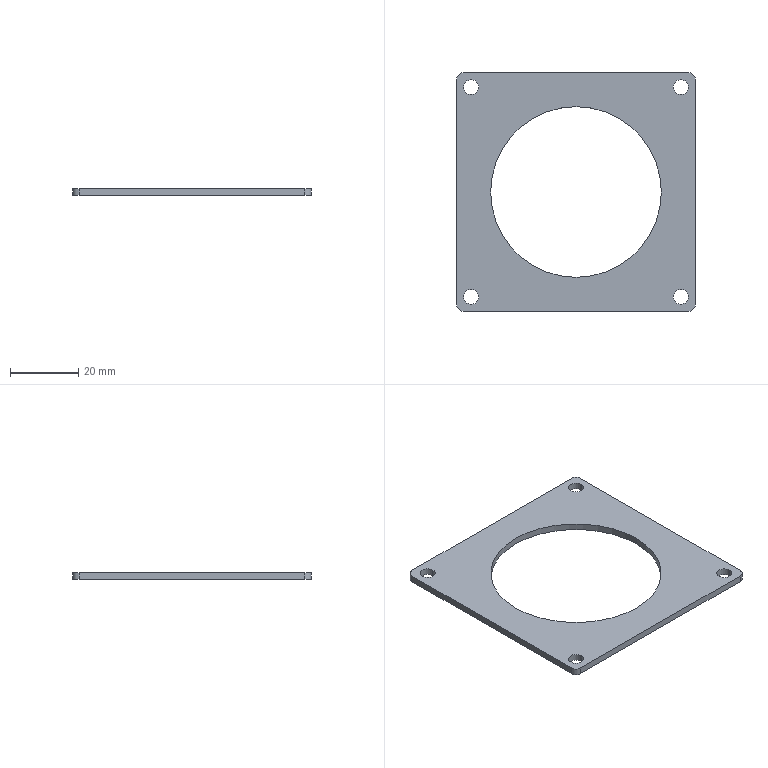Part | SolidWorks | features Cut 2, FlatPattern 1, SMBaseFlange 1, SheetMetal 1 | 1 solid | 20 faces | box 70 x 70 x 2 mm | volume 5744 mm3 | cylinder 14 | plane 6 | commonest cylinder face diameters 4.4 x8 4 x4 50 x2
STEP:
#1=CARTESIAN_POINT('',(-25.,0.,2.));
#2=VERTEX_POINT('',#1);
#3=CARTESIAN_POINT('',(25.,0.,2.));
#4=VERTEX_POINT('',#3);
#5=CARTESIAN_POINT('',(0.,0.,2.));
#6=DIRECTION('',(0.,0.,1.));
#7=DIRECTION('',(1.,0.,0.));
#8=AXIS2_PLACEMENT_3D('',#5,#6,#7);
#9=CIRCLE('',#8,25.);
#10=EDGE_CURVE('',#2,#4,#9,.T.);
#11=ORIENTED_EDGE('',*,*,#10,.T.);
#12=CARTESIAN_POINT('',(25.,0.,0.));
#13=VERTEX_POINT('',#12);
#14=CARTESIAN_POINT('',(25.,0.,10.));
#15=DIRECTION('',(0.,0.,-1.));
#16=VECTOR('',#15,1000.);
#17=LINE('',#14,#16);
#18=EDGE_CURVE('',#4,#13,#17,.T.);
#19=ORIENTED_EDGE('',*,*,#18,.T.);
#20=CARTESIAN_POINT('',(-25.,0.,0.));
#21=VERTEX_POINT('',#20);
#22=CARTESIAN_POINT('',(0.,0.,0.));
#23=DIRECTION('',(0.,0.,-1.));
#24=DIRECTION('',(-1.,0.,0.));
#25=AXIS2_PLACEMENT_3D('',#22,#23,#24);
#26=CIRCLE('',#25,25.);
#27=EDGE_CURVE('',#13,#21,#26,.T.);
#28=ORIENTED_EDGE('',*,*,#27,.T.);
#29=CARTESIAN_POINT('',(-25.,0.,10.));
#30=DIRECTION('',(0.,0.,-1.));
#31=VECTOR('',#30,1000.);
#32=LINE('',#29,#31);
#33=EDGE_CURVE('',#2,#21,#32,.T.);
#34=ORIENTED_EDGE('',*,*,#33,.F.);
#35=EDGE_LOOP('',(#11,#19,#28,#34));
#36=FACE_OUTER_BOUND('',#35,.T.);
#37=CARTESIAN_POINT('',(0.,0.,10.));
#38=DIRECTION('',(0.,0.,-1.));
#39=DIRECTION('',(-1.,0.,0.));
#40=AXIS2_PLACEMENT_3D('',#37,#38,#39);
#41=CYLINDRICAL_SURFACE('',#40,25.);
#42=ADVANCED_FACE('',(#36),#41,.F.);
#43=CARTESIAN_POINT('',(28.55,-30.75,2.));
#44=VERTEX_POINT('',#43);
#45=CARTESIAN_POINT('',(32.95,-30.75,2.));
#46=VERTEX_POINT('',#45);
#47=CARTESIAN_POINT('',(30.75,-30.75,2.));
#48=DIRECTION('',(0.,0.,1.));
#49=DIRECTION('',(1.,0.,0.));
#50=AXIS2_PLACEMENT_3D('',#47,#48,#49);
#51=CIRCLE('',#50,2.2);
#52=EDGE_CURVE('',#44,#46,#51,.T.);
#53=ORIENTED_EDGE('',*,*,#52,.T.);
#54=CARTESIAN_POINT('',(32.95,-30.75,0.));
#55=VERTEX_POINT('',#54);
#56=CARTESIAN_POINT('',(32.95,-30.75,10.));
#57=DIRECTION('',(0.,0.,-1.));
#58=VECTOR('',#57,1000.);
#59=LINE('',#56,#58);
#60=EDGE_CURVE('',#46,#55,#59,.T.);
#61=ORIENTED_EDGE('',*,*,#60,.T.);
#62=CARTESIAN_POINT('',(28.55,-30.75,0.));
#63=VERTEX_POINT('',#62);
#64=CARTESIAN_POINT('',(30.75,-30.75,0.));
#65=DIRECTION('',(0.,0.,-1.));
#66=DIRECTION('',(-1.,0.,0.));
#67=AXIS2_PLACEMENT_3D('',#64,#65,#66);
#68=CIRCLE('',#67,2.2);
#69=EDGE_CURVE('',#55,#63,#68,.T.);
#70=ORIENTED_EDGE('',*,*,#69,.T.);
#71=CARTESIAN_POINT('',(28.55,-30.75,10.));
#72=DIRECTION('',(0.,0.,-1.));
#73=VECTOR('',#72,1000.);
#74=LINE('',#71,#73);
#75=EDGE_CURVE('',#44,#63,#74,.T.);
#76=ORIENTED_EDGE('',*,*,#75,.F.);
#77=EDGE_LOOP('',(#53,#61,#70,#76));
#78=FACE_OUTER_BOUND('',#77,.T.);
#79=CARTESIAN_POINT('',(30.75,-30.75,10.));
#80=DIRECTION('',(0.,0.,-1.));
#81=DIRECTION('',(-1.,0.,0.));
#82=AXIS2_PLACEMENT_3D('',#79,#80,#81);
#83=CYLINDRICAL_SURFACE('',#82,2.2);
#84=ADVANCED_FACE('',(#78),#83,.F.);
#85=CARTESIAN_POINT('',(28.55,30.75,2.));
#86=VERTEX_POINT('',#85);
#87=CARTESIAN_POINT('',(32.95,30.75,2.));
#88=VERTEX_POINT('',#87);
#89=CARTESIAN_POINT('',(30.75,30.75,2.));
#90=DIRECTION('',(0.,0.,1.));
#91=DIRECTION('',(1.,0.,0.));
#92=AXIS2_PLACEMENT_3D('',#89,#90,#91);
#93=CIRCLE('',#92,2.2);
#94=EDGE_CURVE('',#86,#88,#93,.T.);
#95=ORIENTED_EDGE('',*,*,#94,.T.);
#96=CARTESIAN_POINT('',(32.95,30.75,0.));
#97=VERTEX_POINT('',#96);
#98=CARTESIAN_POINT('',(32.95,30.75,10.));
#99=DIRECTION('',(0.,0.,-1.));
#100=VECTOR('',#99,1000.);
#101=LINE('',#98,#100);
#102=EDGE_CURVE('',#88,#97,#101,.T.);
#103=ORIENTED_EDGE('',*,*,#102,.T.);
#104=CARTESIAN_POINT('',(28.55,30.75,0.));
#105=VERTEX_POINT('',#104);
#106=CARTESIAN_POINT('',(30.75,30.75,0.));
#107=DIRECTION('',(0.,0.,-1.));
#108=DIRECTION('',(-1.,0.,0.));
#109=AXIS2_PLACEMENT_3D('',#106,#107,#108);
#110=CIRCLE('',#109,2.2);
#111=EDGE_CURVE('',#97,#105,#110,.T.);
#112=ORIENTED_EDGE('',*,*,#111,.T.);
#113=CARTESIAN_POINT('',(28.55,30.75,10.));
#114=DIRECTION('',(0.,0.,-1.));
#115=VECTOR('',#114,1000.);
#116=LINE('',#113,#115);
#117=EDGE_CURVE('',#86,#105,#116,.T.);
#118=ORIENTED_EDGE('',*,*,#117,.F.);
#119=EDGE_LOOP('',(#95,#103,#112,#118));
#120=FACE_OUTER_BOUND('',#119,.T.);
#121=CARTESIAN_POINT('',(30.75,30.75,10.));
#122=DIRECTION('',(0.,0.,-1.));
#123=DIRECTION('',(-1.,0.,0.));
#124=AXIS2_PLACEMENT_3D('',#121,#122,#123);
#125=CYLINDRICAL_SURFACE('',#124,2.2);
#126=ADVANCED_FACE('',(#120),#125,.F.);
#127=CARTESIAN_POINT('',(-32.95,30.75,2.));
#128=VERTEX_POINT('',#127);
#129=CARTESIAN_POINT('',(-28.55,30.75,2.));
#130=VERTEX_POINT('',#129);
#131=CARTESIAN_POINT('',(-30.75,30.75,2.));
#132=DIRECTION('',(0.,0.,1.));
#133=DIRECTION('',(1.,0.,0.));
#134=AXIS2_PLACEMENT_3D('',#131,#132,#133);
#135=CIRCLE('',#134,2.2);
#136=EDGE_CURVE('',#128,#130,#135,.T.);
#137=ORIENTED_EDGE('',*,*,#136,.T.);
#138=CARTESIAN_POINT('',(-28.55,30.75,0.));
#139=VERTEX_POINT('',#138);
#140=CARTESIAN_POINT('',(-28.55,30.75,10.));
#141=DIRECTION('',(0.,0.,-1.));
#142=VECTOR('',#141,1000.);
#143=LINE('',#140,#142);
#144=EDGE_CURVE('',#130,#139,#143,.T.);
#145=ORIENTED_EDGE('',*,*,#144,.T.);
#146=CARTESIAN_POINT('',(-32.95,30.75,0.));
#147=VERTEX_POINT('',#146);
#148=CARTESIAN_POINT('',(-30.75,30.75,0.));
#149=DIRECTION('',(0.,0.,-1.));
#150=DIRECTION('',(-1.,0.,0.));
#151=AXIS2_PLACEMENT_3D('',#148,#149,#150);
#152=CIRCLE('',#151,2.2);
#153=EDGE_CURVE('',#139,#147,#152,.T.);
#154=ORIENTED_EDGE('',*,*,#153,.T.);
#155=CARTESIAN_POINT('',(-32.95,30.75,10.));
#156=DIRECTION('',(0.,0.,-1.));
#157=VECTOR('',#156,1000.);
#158=LINE('',#155,#157);
#159=EDGE_CURVE('',#128,#147,#158,.T.);
#160=ORIENTED_EDGE('',*,*,#159,.F.);
#161=EDGE_LOOP('',(#137,#145,#154,#160));
#162=FACE_OUTER_BOUND('',#161,.T.);
#163=CARTESIAN_POINT('',(-30.75,30.75,10.));
#164=DIRECTION('',(0.,0.,-1.));
#165=DIRECTION('',(-1.,0.,0.));
#166=AXIS2_PLACEMENT_3D('',#163,#164,#165);
#167=CYLINDRICAL_SURFACE('',#166,2.2);
#168=ADVANCED_FACE('',(#162),#167,.F.);
#169=CARTESIAN_POINT('',(-32.95,-30.75,2.));
#170=VERTEX_POINT('',#169);
#171=CARTESIAN_POINT('',(-28.55,-30.75,2.));
#172=VERTEX_POINT('',#171);
#173=CARTESIAN_POINT('',(-30.75,-30.75,2.));
#174=DIRECTION('',(0.,0.,1.));
#175=DIRECTION('',(1.,0.,0.));
#176=AXIS2_PLACEMENT_3D('',#173,#174,#175);
#177=CIRCLE('',#176,2.2);
#178=EDGE_CURVE('',#170,#172,#177,.T.);
#179=ORIENTED_EDGE('',*,*,#178,.T.);
#180=CARTESIAN_POINT('',(-28.55,-30.75,0.));
#181=VERTEX_POINT('',#180);
#182=CARTESIAN_POINT('',(-28.55,-30.75,10.));
#183=DIRECTION('',(0.,0.,-1.));
#184=VECTOR('',#183,1000.);
#185=LINE('',#182,#184);
#186=EDGE_CURVE('',#172,#181,#185,.T.);
#187=ORIENTED_EDGE('',*,*,#186,.T.);
#188=CARTESIAN_POINT('',(-32.95,-30.75,0.));
#189=VERTEX_POINT('',#188);
#190=CARTESIAN_POINT('',(-30.75,-30.75,0.));
#191=DIRECTION('',(0.,0.,-1.));
#192=DIRECTION('',(-1.,0.,0.));
#193=AXIS2_PLACEMENT_3D('',#190,#191,#192);
#194=CIRCLE('',#193,2.2);
#195=EDGE_CURVE('',#181,#189,#194,.T.);
#196=ORIENTED_EDGE('',*,*,#195,.T.);
#197=CARTESIAN_POINT('',(-32.95,-30.75,10.));
#198=DIRECTION('',(0.,0.,-1.));
#199=VECTOR('',#198,1000.);
#200=LINE('',#197,#199);
#201=EDGE_CURVE('',#170,#189,#200,.T.);
#202=ORIENTED_EDGE('',*,*,#201,.F.);
#203=EDGE_LOOP('',(#179,#187,#196,#202));
#204=FACE_OUTER_BOUND('',#203,.T.);
#205=CARTESIAN_POINT('',(-30.75,-30.75,10.));
#206=DIRECTION('',(0.,0.,-1.));
#207=DIRECTION('',(-1.,0.,0.));
#208=AXIS2_PLACEMENT_3D('',#205,#206,#207);
#209=CYLINDRICAL_SURFACE('',#208,2.2);
#210=ADVANCED_FACE('',(#204),#209,.F.);
#211=CARTESIAN_POINT('',(-35.,-33.,0.));
#212=VERTEX_POINT('',#211);
#213=CARTESIAN_POINT('',(-33.,-35.,0.));
#214=VERTEX_POINT('',#213);
#215=CARTESIAN_POINT('',(-33.,-33.,0.));
#216=DIRECTION('',(0.,0.,1.));
#217=DIRECTION('',(1.,0.,0.));
#218=AXIS2_PLACEMENT_3D('',#215,#216,#217);
#219=CIRCLE('',#218,2.);
#220=EDGE_CURVE('',#212,#214,#219,.T.);
#221=ORIENTED_EDGE('',*,*,#220,.T.);
#222=CARTESIAN_POINT('',(-33.,-35.,2.));
#223=VERTEX_POINT('',#222);
#224=CARTESIAN_POINT('',(-33.,-35.,2.));
#225=DIRECTION('',(0.,0.,-1.));
#226=VECTOR('',#225,1000.);
#227=LINE('',#224,#226);
#228=EDGE_CURVE('',#223,#214,#227,.T.);
#229=ORIENTED_EDGE('',*,*,#228,.F.);
#230=CARTESIAN_POINT('',(-35.,-33.,2.));
#231=VERTEX_POINT('',#230);
#232=CARTESIAN_POINT('',(-33.,-33.,2.));
#233=DIRECTION('',(0.,0.,1.));
#234=DIRECTION('',(1.,0.,0.));
#235=AXIS2_PLACEMENT_3D('',#232,#233,#234);
#236=CIRCLE('',#235,2.);
#237=EDGE_CURVE('',#231,#223,#236,.T.);
#238=ORIENTED_EDGE('',*,*,#237,.F.);
#239=CARTESIAN_POINT('',(-35.,-33.,2.));
#240=DIRECTION('',(0.,0.,-1.));
#241=VECTOR('',#240,1000.);
#242=LINE('',#239,#241);
#243=EDGE_CURVE('',#231,#212,#242,.T.);
#244=ORIENTED_EDGE('',*,*,#243,.T.);
#245=EDGE_LOOP('',(#221,#229,#238,#244));
#246=FACE_OUTER_BOUND('',#245,.T.);
#247=CARTESIAN_POINT('',(-33.,-33.,2.));
#248=DIRECTION('',(0.,0.,-1.));
#249=DIRECTION('',(-1.,0.,0.));
#250=AXIS2_PLACEMENT_3D('',#247,#248,#249);
#251=CYLINDRICAL_SURFACE('',#250,2.);
#252=ADVANCED_FACE('',(#246),#251,.T.);
#253=CARTESIAN_POINT('',(33.,-35.,0.));
#254=VERTEX_POINT('',#253);
#255=CARTESIAN_POINT('',(33.,-35.,0.));
#256=DIRECTION('',(1.,0.,0.));
#257=VECTOR('',#256,1000.);
#258=LINE('',#255,#257);
#259=EDGE_CURVE('',#214,#254,#258,.T.);
#260=ORIENTED_EDGE('',*,*,#259,.T.);
#261=CARTESIAN_POINT('',(33.,-35.,2.));
#262=VERTEX_POINT('',#261);
#263=CARTESIAN_POINT('',(33.,-35.,2.));
#264=DIRECTION('',(0.,0.,-1.));
#265=VECTOR('',#264,1000.);
#266=LINE('',#263,#265);
#267=EDGE_CURVE('',#262,#254,#266,.T.);
#268=ORIENTED_EDGE('',*,*,#267,.F.);
#269=CARTESIAN_POINT('',(33.,-35.,2.));
#270=DIRECTION('',(1.,0.,0.));
#271=VECTOR('',#270,1000.);
#272=LINE('',#269,#271);
#273=EDGE_CURVE('',#223,#262,#272,.T.);
#274=ORIENTED_EDGE('',*,*,#273,.F.);
#275=ORIENTED_EDGE('',*,*,#228,.T.);
#276=EDGE_LOOP('',(#260,#268,#274,#275));
#277=FACE_OUTER_BOUND('',#276,.T.);
#278=CARTESIAN_POINT('',(33.,-35.,2.));
#279=DIRECTION('',(0.,1.,0.));
#280=DIRECTION('',(0.,0.,1.));
#281=AXIS2_PLACEMENT_3D('',#278,#279,#280);
#282=PLANE('',#281);
#283=ADVANCED_FACE('',(#277),#282,.F.);
#284=CARTESIAN_POINT('',(35.,-33.,0.));
#285=VERTEX_POINT('',#284);
#286=CARTESIAN_POINT('',(33.,-33.,0.));
#287=DIRECTION('',(0.,0.,1.));
#288=DIRECTION('',(1.,0.,0.));
#289=AXIS2_PLACEMENT_3D('',#286,#287,#288);
#290=CIRCLE('',#289,2.);
#291=EDGE_CURVE('',#254,#285,#290,.T.);
#292=ORIENTED_EDGE('',*,*,#291,.T.);
#293=CARTESIAN_POINT('',(35.,-33.,2.));
#294=VERTEX_POINT('',#293);
#295=CARTESIAN_POINT('',(35.,-33.,2.));
#296=DIRECTION('',(0.,0.,-1.));
#297=VECTOR('',#296,1000.);
#298=LINE('',#295,#297);
#299=EDGE_CURVE('',#294,#285,#298,.T.);
#300=ORIENTED_EDGE('',*,*,#299,.F.);
#301=CARTESIAN_POINT('',(33.,-33.,2.));
#302=DIRECTION('',(0.,0.,1.));
#303=DIRECTION('',(1.,0.,0.));
#304=AXIS2_PLACEMENT_3D('',#301,#302,#303);
#305=CIRCLE('',#304,2.);
#306=EDGE_CURVE('',#262,#294,#305,.T.);
#307=ORIENTED_EDGE('',*,*,#306,.F.);
#308=ORIENTED_EDGE('',*,*,#267,.T.);
#309=EDGE_LOOP('',(#292,#300,#307,#308));
#310=FACE_OUTER_BOUND('',#309,.T.);
#311=CARTESIAN_POINT('',(33.,-33.,2.));
#312=DIRECTION('',(0.,0.,-1.));
#313=DIRECTION('',(-1.,0.,0.));
#314=AXIS2_PLACEMENT_3D('',#311,#312,#313);
#315=CYLINDRICAL_SURFACE('',#314,2.);
#316=ADVANCED_FACE('',(#310),#315,.T.);
#317=CARTESIAN_POINT('',(35.,33.,0.));
#318=VERTEX_POINT('',#317);
#319=CARTESIAN_POINT('',(35.,33.,0.));
#320=DIRECTION('',(0.,1.,0.));
#321=VECTOR('',#320,1000.);
#322=LINE('',#319,#321);
#323=EDGE_CURVE('',#285,#318,#322,.T.);
#324=ORIENTED_EDGE('',*,*,#323,.T.);
#325=CARTESIAN_POINT('',(35.,33.,2.));
#326=VERTEX_POINT('',#325);
#327=CARTESIAN_POINT('',(35.,33.,2.));
#328=DIRECTION('',(0.,0.,-1.));
#329=VECTOR('',#328,1000.);
#330=LINE('',#327,#329);
#331=EDGE_CURVE('',#326,#318,#330,.T.);
#332=ORIENTED_EDGE('',*,*,#331,.F.);
#333=CARTESIAN_POINT('',(35.,33.,2.));
#334=DIRECTION('',(0.,1.,0.));
#335=VECTOR('',#334,1000.);
#336=LINE('',#333,#335);
#337=EDGE_CURVE('',#294,#326,#336,.T.);
#338=ORIENTED_EDGE('',*,*,#337,.F.);
#339=ORIENTED_EDGE('',*,*,#299,.T.);
#340=EDGE_LOOP('',(#324,#332,#338,#339));
#341=FACE_OUTER_BOUND('',#340,.T.);
#342=CARTESIAN_POINT('',(35.,33.,2.));
#343=DIRECTION('',(-1.,0.,0.));
#344=DIRECTION('',(0.,0.,1.));
#345=AXIS2_PLACEMENT_3D('',#342,#343,#344);
#346=PLANE('',#345);
#347=ADVANCED_FACE('',(#341),#346,.F.);
#348=CARTESIAN_POINT('',(33.,35.,0.));
#349=VERTEX_POINT('',#348);
#350=CARTESIAN_POINT('',(33.,33.,0.));
#351=DIRECTION('',(0.,0.,1.));
#352=DIRECTION('',(1.,0.,0.));
#353=AXIS2_PLACEMENT_3D('',#350,#351,#352);
#354=CIRCLE('',#353,2.);
#355=EDGE_CURVE('',#318,#349,#354,.T.);
#356=ORIENTED_EDGE('',*,*,#355,.T.);
#357=CARTESIAN_POINT('',(33.,35.,2.));
#358=VERTEX_POINT('',#357);
#359=CARTESIAN_POINT('',(33.,35.,2.));
#360=DIRECTION('',(0.,0.,-1.));
#361=VECTOR('',#360,1000.);
#362=LINE('',#359,#361);
#363=EDGE_CURVE('',#358,#349,#362,.T.);
#364=ORIENTED_EDGE('',*,*,#363,.F.);
#365=CARTESIAN_POINT('',(33.,33.,2.));
#366=DIRECTION('',(0.,0.,1.));
#367=DIRECTION('',(1.,0.,0.));
#368=AXIS2_PLACEMENT_3D('',#365,#366,#367);
#369=CIRCLE('',#368,2.);
#370=EDGE_CURVE('',#326,#358,#369,.T.);
#371=ORIENTED_EDGE('',*,*,#370,.F.);
#372=ORIENTED_EDGE('',*,*,#331,.T.);
#373=EDGE_LOOP('',(#356,#364,#371,#372));
#374=FACE_OUTER_BOUND('',#373,.T.);
#375=CARTESIAN_POINT('',(33.,33.,2.));
#376=DIRECTION('',(0.,0.,-1.));
#377=DIRECTION('',(-1.,0.,0.));
#378=AXIS2_PLACEMENT_3D('',#375,#376,#377);
#379=CYLINDRICAL_SURFACE('',#378,2.);
#380=ADVANCED_FACE('',(#374),#379,.T.);
#381=CARTESIAN_POINT('',(-33.,35.,0.));
#382=VERTEX_POINT('',#381);
#383=CARTESIAN_POINT('',(-33.,35.,0.));
#384=DIRECTION('',(-1.,0.,0.));
#385=VECTOR('',#384,1000.);
#386=LINE('',#383,#385);
#387=EDGE_CURVE('',#349,#382,#386,.T.);
#388=ORIENTED_EDGE('',*,*,#387,.T.);
#389=CARTESIAN_POINT('',(-33.,35.,2.));
#390=VERTEX_POINT('',#389);
#391=CARTESIAN_POINT('',(-33.,35.,2.));
#392=DIRECTION('',(0.,0.,-1.));
#393=VECTOR('',#392,1000.);
#394=LINE('',#391,#393);
#395=EDGE_CURVE('',#390,#382,#394,.T.);
#396=ORIENTED_EDGE('',*,*,#395,.F.);
#397=CARTESIAN_POINT('',(-33.,35.,2.));
#398=DIRECTION('',(-1.,0.,0.));
#399=VECTOR('',#398,1000.);
#400=LINE('',#397,#399);
#401=EDGE_CURVE('',#358,#390,#400,.T.);
#402=ORIENTED_EDGE('',*,*,#401,.F.);
#403=ORIENTED_EDGE('',*,*,#363,.T.);
#404=EDGE_LOOP('',(#388,#396,#402,#403));
#405=FACE_OUTER_BOUND('',#404,.T.);
#406=CARTESIAN_POINT('',(-33.,35.,2.));
#407=DIRECTION('',(0.,-1.,0.));
#408=DIRECTION('',(0.,0.,-1.));
#409=AXIS2_PLACEMENT_3D('',#406,#407,#408);
#410=PLANE('',#409);
#411=ADVANCED_FACE('',(#405),#410,.F.);
#412=CARTESIAN_POINT('',(-35.,33.,0.));
#413=VERTEX_POINT('',#412);
#414=CARTESIAN_POINT('',(-33.,33.,0.));
#415=DIRECTION('',(0.,0.,1.));
#416=DIRECTION('',(1.,0.,0.));
#417=AXIS2_PLACEMENT_3D('',#414,#415,#416);
#418=CIRCLE('',#417,2.);
#419=EDGE_CURVE('',#382,#413,#418,.T.);
#420=ORIENTED_EDGE('',*,*,#419,.T.);
#421=CARTESIAN_POINT('',(-35.,33.,2.));
#422=VERTEX_POINT('',#421);
#423=CARTESIAN_POINT('',(-35.,33.,2.));
#424=DIRECTION('',(0.,0.,-1.));
#425=VECTOR('',#424,1000.);
#426=LINE('',#423,#425);
#427=EDGE_CURVE('',#422,#413,#426,.T.);
#428=ORIENTED_EDGE('',*,*,#427,.F.);
#429=CARTESIAN_POINT('',(-33.,33.,2.));
#430=DIRECTION('',(0.,0.,1.));
#431=DIRECTION('',(1.,0.,0.));
#432=AXIS2_PLACEMENT_3D('',#429,#430,#431);
#433=CIRCLE('',#432,2.);
#434=EDGE_CURVE('',#390,#422,#433,.T.);
#435=ORIENTED_EDGE('',*,*,#434,.F.);
#436=ORIENTED_EDGE('',*,*,#395,.T.);
#437=EDGE_LOOP('',(#420,#428,#435,#436));
#438=FACE_OUTER_BOUND('',#437,.T.);
#439=CARTESIAN_POINT('',(-33.,33.,2.));
#440=DIRECTION('',(0.,0.,-1.));
#441=DIRECTION('',(-1.,0.,0.));
#442=AXIS2_PLACEMENT_3D('',#439,#440,#441);
#443=CYLINDRICAL_SURFACE('',#442,2.);
#444=ADVANCED_FACE('',(#438),#443,.T.);
#445=CARTESIAN_POINT('',(-35.,-33.,0.));
#446=DIRECTION('',(0.,-1.,0.));
#447=VECTOR('',#446,1000.);
#448=LINE('',#445,#447);
#449=EDGE_CURVE('',#413,#212,#448,.T.);
#450=ORIENTED_EDGE('',*,*,#449,.T.);
#451=ORIENTED_EDGE('',*,*,#243,.F.);
#452=CARTESIAN_POINT('',(-35.,-33.,2.));
#453=DIRECTION('',(0.,-1.,0.));
#454=VECTOR('',#453,1000.);
#455=LINE('',#452,#454);
#456=EDGE_CURVE('',#422,#231,#455,.T.);
#457=ORIENTED_EDGE('',*,*,#456,.F.);
#458=ORIENTED_EDGE('',*,*,#427,.T.);
#459=EDGE_LOOP('',(#450,#451,#457,#458));
#460=FACE_OUTER_BOUND('',#459,.T.);
#461=CARTESIAN_POINT('',(-35.,-33.,2.));
#462=DIRECTION('',(1.,0.,0.));
#463=DIRECTION('',(0.,0.,-1.));
#464=AXIS2_PLACEMENT_3D('',#461,#462,#463);
#465=PLANE('',#464);
#466=ADVANCED_FACE('',(#460),#465,.F.);
#467=ORIENTED_EDGE('',*,*,#10,.F.);
#468=CARTESIAN_POINT('',(0.,0.,2.));
#469=DIRECTION('',(0.,0.,1.));
#470=DIRECTION('',(1.,0.,0.));
#471=AXIS2_PLACEMENT_3D('',#468,#469,#470);
#472=CIRCLE('',#471,25.);
#473=EDGE_CURVE('',#4,#2,#472,.T.);
#474=ORIENTED_EDGE('',*,*,#473,.F.);
#475=EDGE_LOOP('',(#467,#474));
#476=FACE_BOUND('',#475,.T.);
#477=ORIENTED_EDGE('',*,*,#52,.F.);
#478=CARTESIAN_POINT('',(30.75,-30.75,2.));
#479=DIRECTION('',(0.,0.,1.));
#480=DIRECTION('',(1.,0.,0.));
#481=AXIS2_PLACEMENT_3D('',#478,#479,#480);
#482=CIRCLE('',#481,2.2);
#483=EDGE_CURVE('',#46,#44,#482,.T.);
#484=ORIENTED_EDGE('',*,*,#483,.F.);
#485=EDGE_LOOP('',(#477,#484));
#486=FACE_BOUND('',#485,.T.);
#487=ORIENTED_EDGE('',*,*,#94,.F.);
#488=CARTESIAN_POINT('',(30.75,30.75,2.));
#489=DIRECTION('',(0.,0.,1.));
#490=DIRECTION('',(1.,0.,0.));
#491=AXIS2_PLACEMENT_3D('',#488,#489,#490);
#492=CIRCLE('',#491,2.2);
#493=EDGE_CURVE('',#88,#86,#492,.T.);
#494=ORIENTED_EDGE('',*,*,#493,.F.);
#495=EDGE_LOOP('',(#487,#494));
#496=FACE_BOUND('',#495,.T.);
#497=ORIENTED_EDGE('',*,*,#136,.F.);
#498=CARTESIAN_POINT('',(-30.75,30.75,2.));
#499=DIRECTION('',(0.,0.,1.));
#500=DIRECTION('',(1.,0.,0.));
#501=AXIS2_PLACEMENT_3D('',#498,#499,#500);
#502=CIRCLE('',#501,2.2);
#503=EDGE_CURVE('',#130,#128,#502,.T.);
#504=ORIENTED_EDGE('',*,*,#503,.F.);
#505=EDGE_LOOP('',(#497,#504));
#506=FACE_BOUND('',#505,.T.);
#507=ORIENTED_EDGE('',*,*,#178,.F.);
#508=CARTESIAN_POINT('',(-30.75,-30.75,2.));
#509=DIRECTION('',(0.,0.,1.));
#510=DIRECTION('',(1.,0.,0.));
#511=AXIS2_PLACEMENT_3D('',#508,#509,#510);
#512=CIRCLE('',#511,2.2);
#513=EDGE_CURVE('',#172,#170,#512,.T.);
#514=ORIENTED_EDGE('',*,*,#513,.F.);
#515=EDGE_LOOP('',(#507,#514));
#516=FACE_BOUND('',#515,.T.);
#517=ORIENTED_EDGE('',*,*,#237,.T.);
#518=ORIENTED_EDGE('',*,*,#273,.T.);
#519=ORIENTED_EDGE('',*,*,#306,.T.);
#520=ORIENTED_EDGE('',*,*,#337,.T.);
#521=ORIENTED_EDGE('',*,*,#370,.T.);
#522=ORIENTED_EDGE('',*,*,#401,.T.);
#523=ORIENTED_EDGE('',*,*,#434,.T.);
#524=ORIENTED_EDGE('',*,*,#456,.T.);
#525=EDGE_LOOP('',(#517,#518,#519,#520,#521,#522,#523,#524));
#526=FACE_OUTER_BOUND('',#525,.T.);
#527=CARTESIAN_POINT('',(-33.,-33.,2.));
#528=DIRECTION('',(0.,0.,1.));
#529=DIRECTION('',(1.,0.,0.));
#530=AXIS2_PLACEMENT_3D('',#527,#528,#529);
#531=PLANE('',#530);
#532=ADVANCED_FACE('',(#476,#486,#496,#506,#516,#526),#531,.T.);
#533=CARTESIAN_POINT('',(0.,0.,0.));
#534=DIRECTION('',(0.,0.,-1.));
#535=DIRECTION('',(-1.,0.,0.));
#536=AXIS2_PLACEMENT_3D('',#533,#534,#535);
#537=CIRCLE('',#536,25.);
#538=EDGE_CURVE('',#21,#13,#537,.T.);
#539=ORIENTED_EDGE('',*,*,#538,.F.);
#540=ORIENTED_EDGE('',*,*,#27,.F.);
#541=EDGE_LOOP('',(#539,#540));
#542=FACE_BOUND('',#541,.T.);
#543=CARTESIAN_POINT('',(30.75,-30.75,0.));
#544=DIRECTION('',(0.,0.,-1.));
#545=DIRECTION('',(-1.,0.,0.));
#546=AXIS2_PLACEMENT_3D('',#543,#544,#545);
#547=CIRCLE('',#546,2.2);
#548=EDGE_CURVE('',#63,#55,#547,.T.);
#549=ORIENTED_EDGE('',*,*,#548,.F.);
#550=ORIENTED_EDGE('',*,*,#69,.F.);
#551=EDGE_LOOP('',(#549,#550));
#552=FACE_BOUND('',#551,.T.);
#553=CARTESIAN_POINT('',(30.75,30.75,0.));
#554=DIRECTION('',(0.,0.,-1.));
#555=DIRECTION('',(-1.,0.,0.));
#556=AXIS2_PLACEMENT_3D('',#553,#554,#555);
#557=CIRCLE('',#556,2.2);
#558=EDGE_CURVE('',#105,#97,#557,.T.);
#559=ORIENTED_EDGE('',*,*,#558,.F.);
#560=ORIENTED_EDGE('',*,*,#111,.F.);
#561=EDGE_LOOP('',(#559,#560));
#562=FACE_BOUND('',#561,.T.);
#563=CARTESIAN_POINT('',(-30.75,30.75,0.));
#564=DIRECTION('',(0.,0.,-1.));
#565=DIRECTION('',(-1.,0.,0.));
#566=AXIS2_PLACEMENT_3D('',#563,#564,#565);
#567=CIRCLE('',#566,2.2);
#568=EDGE_CURVE('',#147,#139,#567,.T.);
#569=ORIENTED_EDGE('',*,*,#568,.F.);
#570=ORIENTED_EDGE('',*,*,#153,.F.);
#571=EDGE_LOOP('',(#569,#570));
#572=FACE_BOUND('',#571,.T.);
#573=CARTESIAN_POINT('',(-30.75,-30.75,0.));
#574=DIRECTION('',(0.,0.,-1.));
#575=DIRECTION('',(-1.,0.,0.));
#576=AXIS2_PLACEMENT_3D('',#573,#574,#575);
#577=CIRCLE('',#576,2.2);
#578=EDGE_CURVE('',#189,#181,#577,.T.);
#579=ORIENTED_EDGE('',*,*,#578,.F.);
#580=ORIENTED_EDGE('',*,*,#195,.F.);
#581=EDGE_LOOP('',(#579,#580));
#582=FACE_BOUND('',#581,.T.);
#583=ORIENTED_EDGE('',*,*,#220,.F.);
#584=ORIENTED_EDGE('',*,*,#449,.F.);
#585=ORIENTED_EDGE('',*,*,#419,.F.);
#586=ORIENTED_EDGE('',*,*,#387,.F.);
#587=ORIENTED_EDGE('',*,*,#355,.F.);
#588=ORIENTED_EDGE('',*,*,#323,.F.);
#589=ORIENTED_EDGE('',*,*,#291,.F.);
#590=ORIENTED_EDGE('',*,*,#259,.F.);
#591=EDGE_LOOP('',(#583,#584,#585,#586,#587,#588,#589,#590));
#592=FACE_OUTER_BOUND('',#591,.T.);
#593=CARTESIAN_POINT('',(-33.,-33.,0.));
#594=DIRECTION('',(0.,0.,1.));
#595=DIRECTION('',(1.,0.,0.));
#596=AXIS2_PLACEMENT_3D('',#593,#594,#595);
#597=PLANE('',#596);
#598=ADVANCED_FACE('',(#542,#552,#562,#572,#582,#592),#597,.F.);
#599=ORIENTED_EDGE('',*,*,#186,.F.);
#600=ORIENTED_EDGE('',*,*,#513,.T.);
#601=ORIENTED_EDGE('',*,*,#201,.T.);
#602=ORIENTED_EDGE('',*,*,#578,.T.);
#603=EDGE_LOOP('',(#599,#600,#601,#602));
#604=FACE_OUTER_BOUND('',#603,.T.);
#605=CARTESIAN_POINT('',(-30.75,-30.75,10.));
#606=DIRECTION('',(0.,0.,-1.));
#607=DIRECTION('',(-1.,0.,0.));
#608=AXIS2_PLACEMENT_3D('',#605,#606,#607);
#609=CYLINDRICAL_SURFACE('',#608,2.2);
#610=ADVANCED_FACE('',(#604),#609,.F.);
#611=ORIENTED_EDGE('',*,*,#144,.F.);
#612=ORIENTED_EDGE('',*,*,#503,.T.);
#613=ORIENTED_EDGE('',*,*,#159,.T.);
#614=ORIENTED_EDGE('',*,*,#568,.T.);
#615=EDGE_LOOP('',(#611,#612,#613,#614));
#616=FACE_OUTER_BOUND('',#615,.T.);
#617=CARTESIAN_POINT('',(-30.75,30.75,10.));
#618=DIRECTION('',(0.,0.,-1.));
#619=DIRECTION('',(-1.,0.,0.));
#620=AXIS2_PLACEMENT_3D('',#617,#618,#619);
#621=CYLINDRICAL_SURFACE('',#620,2.2);
#622=ADVANCED_FACE('',(#616),#621,.F.);
#623=ORIENTED_EDGE('',*,*,#102,.F.);
#624=ORIENTED_EDGE('',*,*,#493,.T.);
#625=ORIENTED_EDGE('',*,*,#117,.T.);
#626=ORIENTED_EDGE('',*,*,#558,.T.);
#627=EDGE_LOOP('',(#623,#624,#625,#626));
#628=FACE_OUTER_BOUND('',#627,.T.);
#629=CARTESIAN_POINT('',(30.75,30.75,10.));
#630=DIRECTION('',(0.,0.,-1.));
#631=DIRECTION('',(-1.,0.,0.));
#632=AXIS2_PLACEMENT_3D('',#629,#630,#631);
#633=CYLINDRICAL_SURFACE('',#632,2.2);
#634=ADVANCED_FACE('',(#628),#633,.F.);
#635=ORIENTED_EDGE('',*,*,#60,.F.);
#636=ORIENTED_EDGE('',*,*,#483,.T.);
#637=ORIENTED_EDGE('',*,*,#75,.T.);
#638=ORIENTED_EDGE('',*,*,#548,.T.);
#639=EDGE_LOOP('',(#635,#636,#637,#638));
#640=FACE_OUTER_BOUND('',#639,.T.);
#641=CARTESIAN_POINT('',(30.75,-30.75,10.));
#642=DIRECTION('',(0.,0.,-1.));
#643=DIRECTION('',(-1.,0.,0.));
#644=AXIS2_PLACEMENT_3D('',#641,#642,#643);
#645=CYLINDRICAL_SURFACE('',#644,2.2);
#646=ADVANCED_FACE('',(#640),#645,.F.);
#647=ORIENTED_EDGE('',*,*,#18,.F.);
#648=ORIENTED_EDGE('',*,*,#473,.T.);
#649=ORIENTED_EDGE('',*,*,#33,.T.);
#650=ORIENTED_EDGE('',*,*,#538,.T.);
#651=EDGE_LOOP('',(#647,#648,#649,#650));
#652=FACE_OUTER_BOUND('',#651,.T.);
#653=CARTESIAN_POINT('',(0.,0.,10.));
#654=DIRECTION('',(0.,0.,-1.));
#655=DIRECTION('',(-1.,0.,0.));
#656=AXIS2_PLACEMENT_3D('',#653,#654,#655);
#657=CYLINDRICAL_SURFACE('',#656,25.);
#658=ADVANCED_FACE('',(#652),#657,.F.);
#659=CLOSED_SHELL('',(#42,#84,#126,#168,#210,#252,#283,#316,#347,#380,#411,#444,#466,#532,#598,#610,#622,#634,#646,#658));
#660=MANIFOLD_SOLID_BREP('',#659);
#661=CARTESIAN_POINT('',(0.,0.,0.));
#662=DIRECTION('',(0.,0.,1.));
#663=DIRECTION('',(1.,0.,0.));
#664=AXIS2_PLACEMENT_3D('',#661,#662,#663);
#665=(LENGTH_UNIT()NAMED_UNIT(*)SI_UNIT(.MILLI.,.METRE.));
#666=UNCERTAINTY_MEASURE_WITH_UNIT(LENGTH_MEASURE(0.00001),#665,'','');
#667=(NAMED_UNIT(*)PLANE_ANGLE_UNIT()SI_UNIT($,.RADIAN.));
#668=(NAMED_UNIT(*)SI_UNIT($,.STERADIAN.)SOLID_ANGLE_UNIT());
#669=(GEOMETRIC_REPRESENTATION_CONTEXT(3)GLOBAL_UNCERTAINTY_ASSIGNED_CONTEXT((#666))GLOBAL_UNIT_ASSIGNED_CONTEXT((#665,#667,#668))REPRESENTATION_CONTEXT('',''));
#670=ADVANCED_BREP_SHAPE_REPRESENTATION('',(#660,#664),#669);